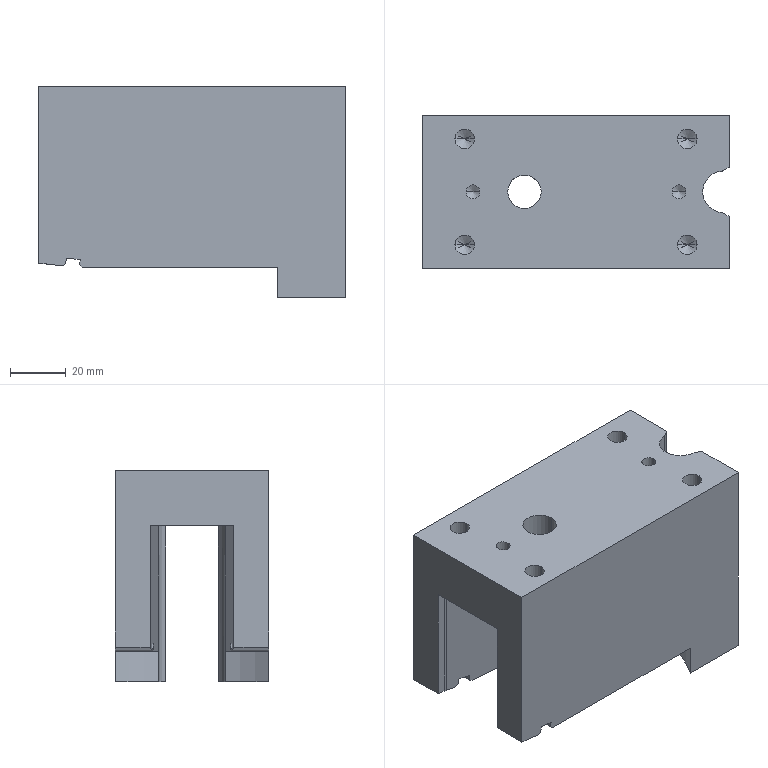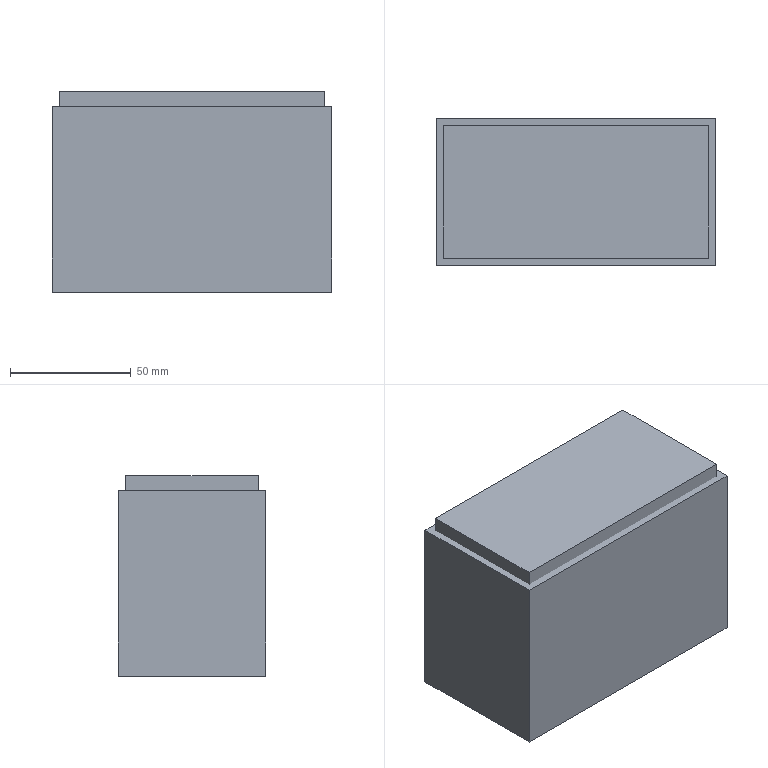CAM job | NX | 3-axis milling, drilling | part box 110 x 55 x 76 mm | stock box 116 x 61 x 83 mm
Tools:
number,name,description,diameter,corner_radius,flute_length,length,flutes
1,D63,Milling Tool-5 Parameters,63.0,0.0,50.0,75.0,2
7,D6A45,Milling Tool-5 Parameters,6.0,0.0,3.0,3.0,2
14,4.8ZT,Drilling Tool,4.8,0.0,35.0,50.0,2
15,5.0JD,Milling Tool-5 Parameters,5.0,0.0,30.0,30.0,4
17,7.0ZT,Drilling Tool,7.0,0.0,35.0,50.0,2
10,D10,Milling Tool-5 Parameters,10.0,0.0,50.0,75.0,2
11,D10JING,Milling Tool-5 Parameters,10.0,0.0,50.0,75.0,2
5,D6R0.5,Milling Tool-5 Parameters,6.0,0.5,50.0,75.0,2
3,D3,Milling Tool-5 Parameters,3.0,0.0,50.0,75.0,2
Operations:
program,operation,operation_type,tool,method,geometry_group,spindle_rpm,surface_speed,feed_per_tooth,feed_cut,feed_plunge,cut_length_mm,path_length_mm,cut_time_min,machine_time_min
1-61-83-116毛胚,FLOOR_WALL,VolumeBased25DMillingOperation,D63,METHOD,A,6500.0,1286.0,0.0962,1250.0,100.0,405.797,459.797,0.3246,0.33
1-61-83-116毛胚,DRILLING_COPY_1,Operation,D6A45,METHOD,A,5000.0,94.0,0.025,250.0,0.0,28.0,302.302,0.112,0.1394
1-61-83-116毛胚,DRILLING_COPY_COPY_1,Operation,4.8ZT,METHOD,A,2000.0,15.0,0.03,120.0,0.0,28.884,194.829,0.2407,0.2573
1-61-83-116毛胚,DRILLING_COPY_COPY_1_COPY,Operation,5.0JD,METHOD,A,1000.0,15.0,0.0125,50.0,0.0,26.0,189.061,0.52,0.5363
1-61-83-116毛胚,DRILLING_COPY_COPY_1_COPY_1,Operation,7.0ZT,METHOD,A,2000.0,15.0,0.03,120.0,0.0,80.412,386.117,0.6701,0.7007
1-61-83-116毛胚,ZLEVEL_PROFILE_COPY_COPY_1_COPY_COPY_COPY,ZLevelMilling,D10,METHOD,A,9500.0,298.0,0.1579,3000.0,1000.0,15011.608,15108.608,5.036,5.045
1-61-83-116毛胚,ZLEVEL_PROFILE_COPY_COPY_1_COPY_COPY_COPY_COPY,ZLevelMilling,D10,METHOD,A,9500.0,298.0,0.1053,2000.0,1000.0,168.748,245.748,0.1083,0.116
1-61-83-116毛胚,ZLEVEL_PROFILE_COPY_COPY_1_COPY_COPY_1,ZLevelMilling,D10JING,METHOD,A,9500.0,298.0,0.0632,1200.0,100.0,760.02,989.714,0.6334,0.6563
1-61-83-116毛胚,ZLEVEL_PROFILE_COPY_COPY_1_COPY_COPY_1_COPY,ZLevelMilling,D10JING,METHOD,A,9500.0,298.0,0.0632,1200.0,100.0,30.755,199.621,0.0256,0.0425
1-61-83-116毛胚,ZLEVEL_PROFILE_1_COPY_1_COPY_COPY,ZLevelMilling,D6A45,METHOD,A,9500.0,179.0,0.0526,1000.0,100.0,503.581,1416.772,0.5036,0.5949
2-61-83-116毛胚,FLOOR_WALL_COPY,VolumeBased25DMillingOperation,D63,METHOD,B,6500.0,1286.0,0.0962,1250.0,100.0,2714.579,3229.363,2.172,2.223
2-61-83-116毛胚,ZLEVEL_PROFILE_COPY_COPY_1_COPY_COPY_COPY_COPY_1,ZLevelMilling,D10,METHOD,B,9500.0,298.0,0.1579,3000.0,1000.0,14638.982,14734.982,4.912,4.921
2-61-83-116毛胚,ADAPTIVE_MILLING,CavityMilling,D10,METHOD,B,9500.0,298.0,0.1579,3000.0,1000.0,25786.554,29961.518,8.62,9.038
2-61-83-116毛胚,FLOOR_WALL_1_COPY,VolumeBased25DMillingOperation,D10JING,METHOD,B,9500.0,179.0,0.0658,1250.0,100.0,754.328,1596.328,0.6035,0.6877
2-61-83-116毛胚,FLOOR_WALL_1,VolumeBased25DMillingOperation,D10JING,METHOD,B,9500.0,179.0,0.0658,1250.0,100.0,1624.293,2742.619,1.299,1.411
2-61-83-116毛胚,ZLEVEL_PROFILE_COPY_COPY_1_COPY_COPY_1_COPY_1,ZLevelMilling,D10JING,METHOD,B,9500.0,298.0,0.0632,1200.0,100.0,760.02,986.714,0.6334,0.656
2-61-83-116毛胚,FIXED_CONTOUR_COPY_COPY_COPY_COPY_1,SurfaceContour,D6R0.5,METHOD,B,9500.0,179.0,0.1579,3000.0,1000.0,5920.43,6090.65,1.979,1.996
2-61-83-116毛胚,ZLEVEL_PROFILE_COPY_1_COPY_1_COPY_1_COPY_COPY,ZLevelMilling,D3,METHOD,B,9500.0,119.0,0.1053,2000.0,800.0,2836.478,3058.052,1.422,1.444
2-61-83-116毛胚,ZLEVEL_PROFILE_COPY_1_COPY_1_COPY_1_COPY_COPY_COPY,ZLevelMilling,D3,METHOD,B,9500.0,119.0,0.1053,2000.0,800.0,1724.401,1915.29,0.8656,0.8847
2-61-83-116毛胚,ZLEVEL_PROFILE_1_COPY_1_COPY_COPY_COPY,ZLevelMilling,D6A45,METHOD,B,9500.0,179.0,0.0526,1000.0,100.0,177.587,361.509,0.1776,0.196
2-61-83-116毛胚,ZLEVEL_PROFILE_1_COPY_1_COPY_COPY_COPY_COPY,ZLevelMilling,D6A45,METHOD,B,9500.0,179.0,0.0526,1000.0,100.0,301.605,730.498,0.3016,0.3445